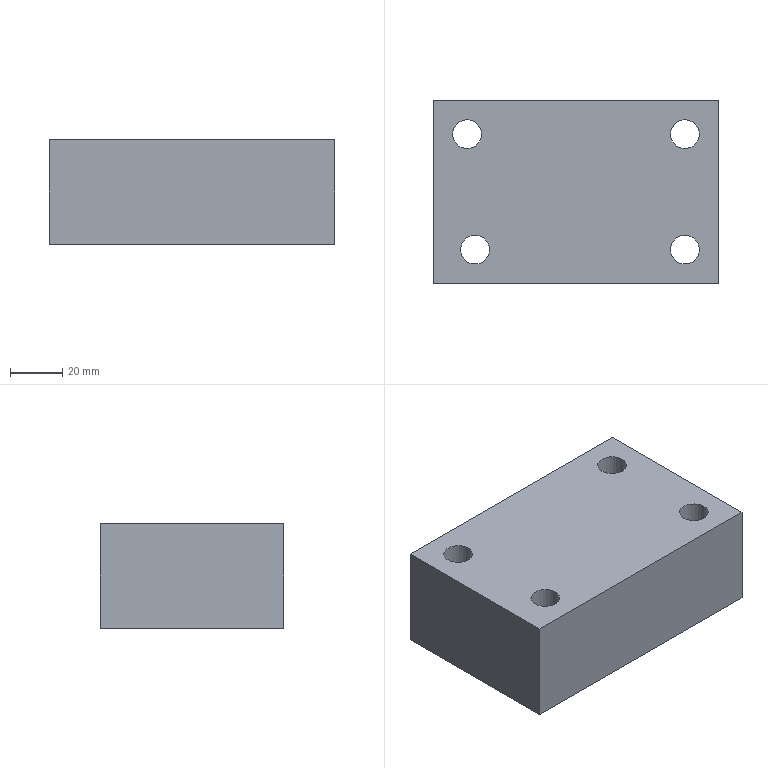Part | STEP file | 119_id1190_x_t | 1 solid | 18 faces | box 109 x 70 x 40 mm | volume 276800 mm3 | plane 10 | cylinder 8 | commonest cylinder face diameters 11 x4 17 x4
STEP:
#1=CARTESIAN_POINT('',(0.,0.,0.));
#2=DIRECTION('',(0.,0.,1.));
#3=DIRECTION('',(1.,0.,0.));
#4=AXIS2_PLACEMENT_3D('',#1,#2,#3);
#5=CARTESIAN_POINT('',(380.5,-156.,65.));
#6=VERTEX_POINT('',#5);
#7=CARTESIAN_POINT('',(380.5,-156.,105.));
#8=VERTEX_POINT('',#7);
#9=CARTESIAN_POINT('',(380.5,-156.,90.));
#10=DIRECTION('',(0.,0.,1.));
#11=VECTOR('',#10,1.);
#12=LINE('',#9,#11);
#13=CARTESIAN_POINT('',(325.,-156.,90.));
#14=DIRECTION('',(0.,-1.,0.));
#15=DIRECTION('',(0.,0.,1.));
#16=AXIS2_PLACEMENT_3D('',#13,#14,#15);
#17=PLANE('',#16);
#18=CARTESIAN_POINT('',(0.,-55.5));
#19=DIRECTION('',(1.,0.));
#20=VECTOR('',#19,1.);
#21=LINE('',#18,#20);
#22=(GEOMETRIC_REPRESENTATION_CONTEXT(2)PARAMETRIC_REPRESENTATION_CONTEXT()REPRESENTATION_CONTEXT('',''));
#23=DEFINITIONAL_REPRESENTATION('',(#21),#22);
#24=PCURVE('',#17,#23);
#25=CARTESIAN_POINT('',(380.5,-122.5,90.));
#26=DIRECTION('',(1.,0.,0.));
#27=DIRECTION('',(0.,0.,1.));
#28=AXIS2_PLACEMENT_3D('',#25,#26,#27);
#29=PLANE('',#28);
#30=CARTESIAN_POINT('',(0.,33.5));
#31=DIRECTION('',(1.,0.));
#32=VECTOR('',#31,1.);
#33=LINE('',#30,#32);
#34=(GEOMETRIC_REPRESENTATION_CONTEXT(2)PARAMETRIC_REPRESENTATION_CONTEXT()REPRESENTATION_CONTEXT('',''));
#35=DEFINITIONAL_REPRESENTATION('',(#33),#34);
#36=PCURVE('',#29,#35);
#37=SURFACE_CURVE('',#12,(#24,#36),.PCURVE_S1.);
#38=EDGE_CURVE('',#6,#8,#37,.T.);
#39=ORIENTED_EDGE('',*,*,#38,.T.);
#40=CARTESIAN_POINT('',(271.5,-156.,105.));
#41=VERTEX_POINT('',#40);
#42=CARTESIAN_POINT('',(325.,-156.,105.));
#43=DIRECTION('',(-1.,0.,0.));
#44=VECTOR('',#43,1.);
#45=LINE('',#42,#44);
#46=CARTESIAN_POINT('',(15.,0.));
#47=DIRECTION('',(0.,1.));
#48=VECTOR('',#47,1.);
#49=LINE('',#46,#48);
#50=(GEOMETRIC_REPRESENTATION_CONTEXT(2)PARAMETRIC_REPRESENTATION_CONTEXT()REPRESENTATION_CONTEXT('',''));
#51=DEFINITIONAL_REPRESENTATION('',(#49),#50);
#52=PCURVE('',#17,#51);
#53=CARTESIAN_POINT('',(325.,-122.5,105.));
#54=DIRECTION('',(0.,0.,1.));
#55=DIRECTION('',(-1.,0.,0.));
#56=AXIS2_PLACEMENT_3D('',#53,#54,#55);
#57=PLANE('',#56);
#58=CARTESIAN_POINT('',(0.,33.5));
#59=DIRECTION('',(1.,0.));
#60=VECTOR('',#59,1.);
#61=LINE('',#58,#60);
#62=(GEOMETRIC_REPRESENTATION_CONTEXT(2)PARAMETRIC_REPRESENTATION_CONTEXT()REPRESENTATION_CONTEXT('',''));
#63=DEFINITIONAL_REPRESENTATION('',(#61),#62);
#64=PCURVE('',#57,#63);
#65=SURFACE_CURVE('',#45,(#52,#64),.PCURVE_S1.);
#66=EDGE_CURVE('',#8,#41,#65,.T.);
#67=ORIENTED_EDGE('',*,*,#66,.T.);
#68=CARTESIAN_POINT('',(271.5,-156.,65.));
#69=VERTEX_POINT('',#68);
#70=CARTESIAN_POINT('',(271.5,-156.,90.));
#71=DIRECTION('',(0.,0.,1.));
#72=VECTOR('',#71,1.);
#73=LINE('',#70,#72);
#74=CARTESIAN_POINT('',(0.,53.5));
#75=DIRECTION('',(1.,0.));
#76=VECTOR('',#75,1.);
#77=LINE('',#74,#76);
#78=(GEOMETRIC_REPRESENTATION_CONTEXT(2)PARAMETRIC_REPRESENTATION_CONTEXT()REPRESENTATION_CONTEXT('',''));
#79=DEFINITIONAL_REPRESENTATION('',(#77),#78);
#80=PCURVE('',#17,#79);
#81=CARTESIAN_POINT('',(271.5,-122.5,90.));
#82=DIRECTION('',(-1.,0.,0.));
#83=DIRECTION('',(0.,0.,-1.));
#84=AXIS2_PLACEMENT_3D('',#81,#82,#83);
#85=PLANE('',#84);
#86=CARTESIAN_POINT('',(0.,33.5));
#87=DIRECTION('',(-1.,0.));
#88=VECTOR('',#87,1.);
#89=LINE('',#86,#88);
#90=(GEOMETRIC_REPRESENTATION_CONTEXT(2)PARAMETRIC_REPRESENTATION_CONTEXT()REPRESENTATION_CONTEXT('',''));
#91=DEFINITIONAL_REPRESENTATION('',(#89),#90);
#92=PCURVE('',#85,#91);
#93=SURFACE_CURVE('',#73,(#80,#92),.PCURVE_S1.);
#94=EDGE_CURVE('',#69,#41,#93,.T.);
#95=ORIENTED_EDGE('',*,*,#94,.F.);
#96=CARTESIAN_POINT('',(325.,-156.,65.));
#97=DIRECTION('',(1.,0.,0.));
#98=VECTOR('',#97,1.);
#99=LINE('',#96,#98);
#100=CARTESIAN_POINT('',(-25.,0.));
#101=DIRECTION('',(0.,-1.));
#102=VECTOR('',#101,1.);
#103=LINE('',#100,#102);
#104=(GEOMETRIC_REPRESENTATION_CONTEXT(2)PARAMETRIC_REPRESENTATION_CONTEXT()REPRESENTATION_CONTEXT('',''));
#105=DEFINITIONAL_REPRESENTATION('',(#103),#104);
#106=PCURVE('',#17,#105);
#107=CARTESIAN_POINT('',(-346.389,-676.223,65.));
#108=DIRECTION('',(0.,0.,-1.));
#109=DIRECTION('',(-1.,0.,0.));
#110=AXIS2_PLACEMENT_3D('',#107,#108,#109);
#111=PLANE('',#110);
#112=CARTESIAN_POINT('',(-671.389,520.223));
#113=DIRECTION('',(-1.,0.));
#114=VECTOR('',#113,1.);
#115=LINE('',#112,#114);
#116=(GEOMETRIC_REPRESENTATION_CONTEXT(2)PARAMETRIC_REPRESENTATION_CONTEXT()REPRESENTATION_CONTEXT('',''));
#117=DEFINITIONAL_REPRESENTATION('',(#115),#116);
#118=PCURVE('',#111,#117);
#119=SURFACE_CURVE('',#99,(#106,#118),.PCURVE_S1.);
#120=EDGE_CURVE('',#69,#6,#119,.T.);
#121=ORIENTED_EDGE('',*,*,#120,.T.);
#122=EDGE_LOOP('',(#39,#67,#95,#121));
#123=FACE_BOUND('',#122,.T.);
#124=ADVANCED_FACE('',(#123),#17,.T.);
#125=ORIENTED_EDGE('',*,*,#94,.T.);
#126=CARTESIAN_POINT('',(271.5,-86.,105.));
#127=VERTEX_POINT('',#126);
#128=CARTESIAN_POINT('',(271.5,-122.5,105.));
#129=DIRECTION('',(0.,1.,0.));
#130=VECTOR('',#129,1.);
#131=LINE('',#128,#130);
#132=CARTESIAN_POINT('',(-15.,0.));
#133=DIRECTION('',(0.,-1.));
#134=VECTOR('',#133,1.);
#135=LINE('',#132,#134);
#136=(GEOMETRIC_REPRESENTATION_CONTEXT(2)PARAMETRIC_REPRESENTATION_CONTEXT()REPRESENTATION_CONTEXT('',''));
#137=DEFINITIONAL_REPRESENTATION('',(#135),#136);
#138=PCURVE('',#85,#137);
#139=CARTESIAN_POINT('',(53.5,0.));
#140=DIRECTION('',(0.,-1.));
#141=VECTOR('',#140,1.);
#142=LINE('',#139,#141);
#143=(GEOMETRIC_REPRESENTATION_CONTEXT(2)PARAMETRIC_REPRESENTATION_CONTEXT()REPRESENTATION_CONTEXT('',''));
#144=DEFINITIONAL_REPRESENTATION('',(#142),#143);
#145=PCURVE('',#57,#144);
#146=SURFACE_CURVE('',#131,(#138,#145),.PCURVE_S1.);
#147=EDGE_CURVE('',#41,#127,#146,.T.);
#148=ORIENTED_EDGE('',*,*,#147,.T.);
#149=CARTESIAN_POINT('',(271.5,-86.,65.));
#150=VERTEX_POINT('',#149);
#151=CARTESIAN_POINT('',(271.5,-86.,90.));
#152=DIRECTION('',(0.,0.,1.));
#153=VECTOR('',#152,1.);
#154=LINE('',#151,#153);
#155=CARTESIAN_POINT('',(0.,-36.5));
#156=DIRECTION('',(-1.,0.));
#157=VECTOR('',#156,1.);
#158=LINE('',#155,#157);
#159=(GEOMETRIC_REPRESENTATION_CONTEXT(2)PARAMETRIC_REPRESENTATION_CONTEXT()REPRESENTATION_CONTEXT('',''));
#160=DEFINITIONAL_REPRESENTATION('',(#158),#159);
#161=PCURVE('',#85,#160);
#162=CARTESIAN_POINT('',(325.,-86.,90.));
#163=DIRECTION('',(0.,1.,0.));
#164=DIRECTION('',(0.,0.,-1.));
#165=AXIS2_PLACEMENT_3D('',#162,#163,#164);
#166=PLANE('',#165);
#167=CARTESIAN_POINT('',(0.,53.5));
#168=DIRECTION('',(-1.,0.));
#169=VECTOR('',#168,1.);
#170=LINE('',#167,#169);
#171=(GEOMETRIC_REPRESENTATION_CONTEXT(2)PARAMETRIC_REPRESENTATION_CONTEXT()REPRESENTATION_CONTEXT('',''));
#172=DEFINITIONAL_REPRESENTATION('',(#170),#171);
#173=PCURVE('',#166,#172);
#174=SURFACE_CURVE('',#154,(#161,#173),.PCURVE_S1.);
#175=EDGE_CURVE('',#150,#127,#174,.T.);
#176=ORIENTED_EDGE('',*,*,#175,.F.);
#177=CARTESIAN_POINT('',(271.5,-122.5,65.));
#178=DIRECTION('',(0.,-1.,0.));
#179=VECTOR('',#178,1.);
#180=LINE('',#177,#179);
#181=CARTESIAN_POINT('',(25.,0.));
#182=DIRECTION('',(0.,1.));
#183=VECTOR('',#182,1.);
#184=LINE('',#181,#183);
#185=(GEOMETRIC_REPRESENTATION_CONTEXT(2)PARAMETRIC_REPRESENTATION_CONTEXT()REPRESENTATION_CONTEXT('',''));
#186=DEFINITIONAL_REPRESENTATION('',(#184),#185);
#187=PCURVE('',#85,#186);
#188=CARTESIAN_POINT('',(-617.889,553.723));
#189=DIRECTION('',(0.,-1.));
#190=VECTOR('',#189,1.);
#191=LINE('',#188,#190);
#192=(GEOMETRIC_REPRESENTATION_CONTEXT(2)PARAMETRIC_REPRESENTATION_CONTEXT()REPRESENTATION_CONTEXT('',''));
#193=DEFINITIONAL_REPRESENTATION('',(#191),#192);
#194=PCURVE('',#111,#193);
#195=SURFACE_CURVE('',#180,(#187,#194),.PCURVE_S1.);
#196=EDGE_CURVE('',#150,#69,#195,.T.);
#197=ORIENTED_EDGE('',*,*,#196,.T.);
#198=EDGE_LOOP('',(#125,#148,#176,#197));
#199=FACE_BOUND('',#198,.T.);
#200=ADVANCED_FACE('',(#199),#85,.T.);
#201=ORIENTED_EDGE('',*,*,#175,.T.);
#202=CARTESIAN_POINT('',(380.5,-86.,105.));
#203=VERTEX_POINT('',#202);
#204=CARTESIAN_POINT('',(325.,-86.,105.));
#205=DIRECTION('',(1.,0.,0.));
#206=VECTOR('',#205,1.);
#207=LINE('',#204,#206);
#208=CARTESIAN_POINT('',(-15.,0.));
#209=DIRECTION('',(0.,-1.));
#210=VECTOR('',#209,1.);
#211=LINE('',#208,#210);
#212=(GEOMETRIC_REPRESENTATION_CONTEXT(2)PARAMETRIC_REPRESENTATION_CONTEXT()REPRESENTATION_CONTEXT('',''));
#213=DEFINITIONAL_REPRESENTATION('',(#211),#212);
#214=PCURVE('',#166,#213);
#215=CARTESIAN_POINT('',(0.,-36.5));
#216=DIRECTION('',(-1.,0.));
#217=VECTOR('',#216,1.);
#218=LINE('',#215,#217);
#219=(GEOMETRIC_REPRESENTATION_CONTEXT(2)PARAMETRIC_REPRESENTATION_CONTEXT()REPRESENTATION_CONTEXT('',''));
#220=DEFINITIONAL_REPRESENTATION('',(#218),#219);
#221=PCURVE('',#57,#220);
#222=SURFACE_CURVE('',#207,(#214,#221),.PCURVE_S1.);
#223=EDGE_CURVE('',#127,#203,#222,.T.);
#224=ORIENTED_EDGE('',*,*,#223,.T.);
#225=CARTESIAN_POINT('',(380.5,-86.,65.));
#226=VERTEX_POINT('',#225);
#227=CARTESIAN_POINT('',(380.5,-86.,90.));
#228=DIRECTION('',(0.,0.,1.));
#229=VECTOR('',#228,1.);
#230=LINE('',#227,#229);
#231=CARTESIAN_POINT('',(0.,-55.5));
#232=DIRECTION('',(-1.,0.));
#233=VECTOR('',#232,1.);
#234=LINE('',#231,#233);
#235=(GEOMETRIC_REPRESENTATION_CONTEXT(2)PARAMETRIC_REPRESENTATION_CONTEXT()REPRESENTATION_CONTEXT('',''));
#236=DEFINITIONAL_REPRESENTATION('',(#234),#235);
#237=PCURVE('',#166,#236);
#238=CARTESIAN_POINT('',(0.,-36.5));
#239=DIRECTION('',(1.,0.));
#240=VECTOR('',#239,1.);
#241=LINE('',#238,#240);
#242=(GEOMETRIC_REPRESENTATION_CONTEXT(2)PARAMETRIC_REPRESENTATION_CONTEXT()REPRESENTATION_CONTEXT('',''));
#243=DEFINITIONAL_REPRESENTATION('',(#241),#242);
#244=PCURVE('',#29,#243);
#245=SURFACE_CURVE('',#230,(#237,#244),.PCURVE_S1.);
#246=EDGE_CURVE('',#226,#203,#245,.T.);
#247=ORIENTED_EDGE('',*,*,#246,.F.);
#248=CARTESIAN_POINT('',(325.,-86.,65.));
#249=DIRECTION('',(-1.,0.,0.));
#250=VECTOR('',#249,1.);
#251=LINE('',#248,#250);
#252=CARTESIAN_POINT('',(25.,0.));
#253=DIRECTION('',(0.,1.));
#254=VECTOR('',#253,1.);
#255=LINE('',#252,#254);
#256=(GEOMETRIC_REPRESENTATION_CONTEXT(2)PARAMETRIC_REPRESENTATION_CONTEXT()REPRESENTATION_CONTEXT('',''));
#257=DEFINITIONAL_REPRESENTATION('',(#255),#256);
#258=PCURVE('',#166,#257);
#259=CARTESIAN_POINT('',(-671.389,590.223));
#260=DIRECTION('',(1.,0.));
#261=VECTOR('',#260,1.);
#262=LINE('',#259,#261);
#263=(GEOMETRIC_REPRESENTATION_CONTEXT(2)PARAMETRIC_REPRESENTATION_CONTEXT()REPRESENTATION_CONTEXT('',''));
#264=DEFINITIONAL_REPRESENTATION('',(#262),#263);
#265=PCURVE('',#111,#264);
#266=SURFACE_CURVE('',#251,(#258,#265),.PCURVE_S1.);
#267=EDGE_CURVE('',#226,#150,#266,.T.);
#268=ORIENTED_EDGE('',*,*,#267,.T.);
#269=EDGE_LOOP('',(#201,#224,#247,#268));
#270=FACE_BOUND('',#269,.T.);
#271=ADVANCED_FACE('',(#270),#166,.T.);
#272=ORIENTED_EDGE('',*,*,#246,.T.);
#273=CARTESIAN_POINT('',(380.5,-122.5,105.));
#274=DIRECTION('',(0.,-1.,0.));
#275=VECTOR('',#274,1.);
#276=LINE('',#273,#275);
#277=CARTESIAN_POINT('',(15.,0.));
#278=DIRECTION('',(0.,1.));
#279=VECTOR('',#278,1.);
#280=LINE('',#277,#279);
#281=(GEOMETRIC_REPRESENTATION_CONTEXT(2)PARAMETRIC_REPRESENTATION_CONTEXT()REPRESENTATION_CONTEXT('',''));
#282=DEFINITIONAL_REPRESENTATION('',(#280),#281);
#283=PCURVE('',#29,#282);
#284=CARTESIAN_POINT('',(-55.5,0.));
#285=DIRECTION('',(0.,1.));
#286=VECTOR('',#285,1.);
#287=LINE('',#284,#286);
#288=(GEOMETRIC_REPRESENTATION_CONTEXT(2)PARAMETRIC_REPRESENTATION_CONTEXT()REPRESENTATION_CONTEXT('',''));
#289=DEFINITIONAL_REPRESENTATION('',(#287),#288);
#290=PCURVE('',#57,#289);
#291=SURFACE_CURVE('',#276,(#283,#290),.PCURVE_S1.);
#292=EDGE_CURVE('',#203,#8,#291,.T.);
#293=ORIENTED_EDGE('',*,*,#292,.T.);
#294=ORIENTED_EDGE('',*,*,#38,.F.);
#295=CARTESIAN_POINT('',(380.5,-122.5,65.));
#296=DIRECTION('',(0.,1.,0.));
#297=VECTOR('',#296,1.);
#298=LINE('',#295,#297);
#299=CARTESIAN_POINT('',(-25.,0.));
#300=DIRECTION('',(0.,-1.));
#301=VECTOR('',#300,1.);
#302=LINE('',#299,#301);
#303=(GEOMETRIC_REPRESENTATION_CONTEXT(2)PARAMETRIC_REPRESENTATION_CONTEXT()REPRESENTATION_CONTEXT('',''));
#304=DEFINITIONAL_REPRESENTATION('',(#302),#303);
#305=PCURVE('',#29,#304);
#306=CARTESIAN_POINT('',(-726.889,553.723));
#307=DIRECTION('',(0.,1.));
#308=VECTOR('',#307,1.);
#309=LINE('',#306,#308);
#310=(GEOMETRIC_REPRESENTATION_CONTEXT(2)PARAMETRIC_REPRESENTATION_CONTEXT()REPRESENTATION_CONTEXT('',''));
#311=DEFINITIONAL_REPRESENTATION('',(#309),#310);
#312=PCURVE('',#111,#311);
#313=SURFACE_CURVE('',#298,(#305,#312),.PCURVE_S1.);
#314=EDGE_CURVE('',#6,#226,#313,.T.);
#315=ORIENTED_EDGE('',*,*,#314,.T.);
#316=EDGE_LOOP('',(#272,#293,#294,#315));
#317=FACE_BOUND('',#316,.T.);
#318=ADVANCED_FACE('',(#317),#29,.T.);
#319=CARTESIAN_POINT('',(279.,-143.,65.));
#320=VERTEX_POINT('',#319);
#321=CARTESIAN_POINT('',(287.5,-143.,65.));
#322=DIRECTION('',(0.,0.,1.));
#323=DIRECTION('',(-1.,0.,0.));
#324=AXIS2_PLACEMENT_3D('',#321,#322,#323);
#325=CIRCLE('',#324,8.5);
#326=CARTESIAN_POINT('',(287.5,-143.,90.));
#327=DIRECTION('',(0.,0.,1.));
#328=DIRECTION('',(-1.,0.,0.));
#329=AXIS2_PLACEMENT_3D('',#326,#327,#328);
#330=CYLINDRICAL_SURFACE('',#329,8.5);
#331=CARTESIAN_POINT('',(0.,-25.));
#332=DIRECTION('',(1.,0.));
#333=VECTOR('',#332,1.);
#334=LINE('',#331,#333);
#335=(GEOMETRIC_REPRESENTATION_CONTEXT(2)PARAMETRIC_REPRESENTATION_CONTEXT()REPRESENTATION_CONTEXT('',''));
#336=DEFINITIONAL_REPRESENTATION('',(#334),#335);
#337=PCURVE('',#330,#336);
#338=CARTESIAN_POINT('',(-625.389,533.223));
#339=CARTESIAN_POINT('',(-625.389,518.5));
#340=CARTESIAN_POINT('',(-638.139,525.862));
#341=CARTESIAN_POINT('',(-650.889,533.223));
#342=CARTESIAN_POINT('',(-638.139,540.584));
#343=CARTESIAN_POINT('',(-625.389,547.945));
#344=CARTESIAN_POINT('',(-625.389,533.223));
#345=(BOUNDED_CURVE()B_SPLINE_CURVE(2,(#338,#339,#340,#341,#342,#343,#344),.UNSPECIFIED.,.T.,.F.)B_SPLINE_CURVE_WITH_KNOTS((1,2,2,2,2,1),(-2.094,0.,2.094,4.189,6.283,8.378),.UNSPECIFIED.)CURVE()GEOMETRIC_REPRESENTATION_ITEM()RATIONAL_B_SPLINE_CURVE((1.,0.5,1.,0.5,1.,0.5,1.))REPRESENTATION_ITEM(''));
#346=(GEOMETRIC_REPRESENTATION_CONTEXT(2)PARAMETRIC_REPRESENTATION_CONTEXT()REPRESENTATION_CONTEXT('',''));
#347=DEFINITIONAL_REPRESENTATION('',(#345),#346);
#348=PCURVE('',#111,#347);
#349=SURFACE_CURVE('',#325,(#337,#348),.PCURVE_S1.);
#350=EDGE_CURVE('',#320,#320,#349,.T.);
#351=ORIENTED_EDGE('',*,*,#350,.T.);
#352=CARTESIAN_POINT('',(279.,-143.,90.));
#353=VERTEX_POINT('',#352);
#354=CARTESIAN_POINT('',(279.,-143.,65.));
#355=CARTESIAN_POINT('',(279.,-143.,90.));
#356=B_SPLINE_CURVE_WITH_KNOTS('',1,(#354,#355),.UNSPECIFIED.,.F.,.F.,(2,2),(-25.,0.),.PIECEWISE_BEZIER_KNOTS.);
#357=CARTESIAN_POINT('',(6.283,0.));
#358=DIRECTION('',(0.,1.));
#359=VECTOR('',#358,1.);
#360=LINE('',#357,#359);
#361=(GEOMETRIC_REPRESENTATION_CONTEXT(2)PARAMETRIC_REPRESENTATION_CONTEXT()REPRESENTATION_CONTEXT('',''));
#362=DEFINITIONAL_REPRESENTATION('',(#360),#361);
#363=PCURVE('',#330,#362);
#364=CARTESIAN_POINT('',(0.,0.));
#365=DIRECTION('',(0.,1.));
#366=VECTOR('',#365,1.);
#367=LINE('',#364,#366);
#368=(GEOMETRIC_REPRESENTATION_CONTEXT(2)PARAMETRIC_REPRESENTATION_CONTEXT()REPRESENTATION_CONTEXT('',''));
#369=DEFINITIONAL_REPRESENTATION('',(#367),#368);
#370=PCURVE('',#330,#369);
#371=SEAM_CURVE('',#356,(#363,#370),.PCURVE_S1.);
#372=EDGE_CURVE('',#320,#353,#371,.T.);
#373=ORIENTED_EDGE('',*,*,#372,.T.);
#374=CARTESIAN_POINT('',(296.,-143.,90.));
#375=VERTEX_POINT('',#374);
#376=CARTESIAN_POINT('',(287.5,-143.,90.));
#377=DIRECTION('',(0.,0.,1.));
#378=DIRECTION('',(1.,0.,0.));
#379=AXIS2_PLACEMENT_3D('',#376,#377,#378);
#380=CIRCLE('',#379,8.5);
#381=CARTESIAN_POINT('',(3.142,0.));
#382=DIRECTION('',(1.,0.));
#383=VECTOR('',#382,1.);
#384=LINE('',#381,#383);
#385=(GEOMETRIC_REPRESENTATION_CONTEXT(2)PARAMETRIC_REPRESENTATION_CONTEXT()REPRESENTATION_CONTEXT('',''));
#386=DEFINITIONAL_REPRESENTATION('',(#384),#385);
#387=PCURVE('',#330,#386);
#388=CARTESIAN_POINT('',(326.,-121.,90.));
#389=DIRECTION('',(0.,0.,1.));
#390=DIRECTION('',(1.,0.,0.));
#391=AXIS2_PLACEMENT_3D('',#388,#389,#390);
#392=PLANE('',#391);
#393=CARTESIAN_POINT('',(-38.5,-22.));
#394=DIRECTION('',(1.,0.));
#395=AXIS2_PLACEMENT_2D('',#393,#394);
#396=CIRCLE('',#395,8.5);
#397=(GEOMETRIC_REPRESENTATION_CONTEXT(2)PARAMETRIC_REPRESENTATION_CONTEXT()REPRESENTATION_CONTEXT('',''));
#398=DEFINITIONAL_REPRESENTATION('',(#396),#397);
#399=PCURVE('',#392,#398);
#400=SURFACE_CURVE('',#380,(#387,#399),.PCURVE_S1.);
#401=EDGE_CURVE('',#375,#353,#400,.T.);
#402=ORIENTED_EDGE('',*,*,#401,.F.);
#403=CARTESIAN_POINT('',(287.5,-143.,90.));
#404=DIRECTION('',(0.,0.,1.));
#405=DIRECTION('',(1.,0.,0.));
#406=AXIS2_PLACEMENT_3D('',#403,#404,#405);
#407=CIRCLE('',#406,8.5);
#408=CARTESIAN_POINT('',(-3.142,0.));
#409=DIRECTION('',(1.,0.));
#410=VECTOR('',#409,1.);
#411=LINE('',#408,#410);
#412=(GEOMETRIC_REPRESENTATION_CONTEXT(2)PARAMETRIC_REPRESENTATION_CONTEXT()REPRESENTATION_CONTEXT('',''));
#413=DEFINITIONAL_REPRESENTATION('',(#411),#412);
#414=PCURVE('',#330,#413);
#415=CARTESIAN_POINT('',(-38.5,-22.));
#416=DIRECTION('',(1.,0.));
#417=AXIS2_PLACEMENT_2D('',#415,#416);
#418=CIRCLE('',#417,8.5);
#419=(GEOMETRIC_REPRESENTATION_CONTEXT(2)PARAMETRIC_REPRESENTATION_CONTEXT()REPRESENTATION_CONTEXT('',''));
#420=DEFINITIONAL_REPRESENTATION('',(#418),#419);
#421=PCURVE('',#392,#420);
#422=SURFACE_CURVE('',#407,(#414,#421),.PCURVE_S1.);
#423=EDGE_CURVE('',#353,#375,#422,.T.);
#424=ORIENTED_EDGE('',*,*,#423,.F.);
#425=ORIENTED_EDGE('',*,*,#372,.F.);
#426=EDGE_LOOP('',(#351,#373,#402,#424,#425));
#427=FACE_BOUND('',#426,.F.);
#428=ADVANCED_FACE('',(#427),#330,.F.);
#429=CARTESIAN_POINT('',(359.,-143.,65.));
#430=VERTEX_POINT('',#429);
#431=CARTESIAN_POINT('',(367.5,-143.,65.));
#432=DIRECTION('',(0.,0.,1.));
#433=DIRECTION('',(-1.,0.,0.));
#434=AXIS2_PLACEMENT_3D('',#431,#432,#433);
#435=CIRCLE('',#434,8.5);
#436=CARTESIAN_POINT('',(367.5,-143.,90.));
#437=DIRECTION('',(0.,0.,1.));
#438=DIRECTION('',(-1.,0.,0.));
#439=AXIS2_PLACEMENT_3D('',#436,#437,#438);
#440=CYLINDRICAL_SURFACE('',#439,8.5);
#441=CARTESIAN_POINT('',(0.,-25.));
#442=DIRECTION('',(1.,0.));
#443=VECTOR('',#442,1.);
#444=LINE('',#441,#443);
#445=(GEOMETRIC_REPRESENTATION_CONTEXT(2)PARAMETRIC_REPRESENTATION_CONTEXT()REPRESENTATION_CONTEXT('',''));
#446=DEFINITIONAL_REPRESENTATION('',(#444),#445);
#447=PCURVE('',#440,#446);
#448=CARTESIAN_POINT('',(-705.389,533.223));
#449=CARTESIAN_POINT('',(-705.389,518.5));
#450=CARTESIAN_POINT('',(-718.139,525.862));
#451=CARTESIAN_POINT('',(-730.889,533.223));
#452=CARTESIAN_POINT('',(-718.139,540.584));
#453=CARTESIAN_POINT('',(-705.389,547.945));
#454=CARTESIAN_POINT('',(-705.389,533.223));
#455=(BOUNDED_CURVE()B_SPLINE_CURVE(2,(#448,#449,#450,#451,#452,#453,#454),.UNSPECIFIED.,.T.,.F.)B_SPLINE_CURVE_WITH_KNOTS((1,2,2,2,2,1),(-2.094,0.,2.094,4.189,6.283,8.378),.UNSPECIFIED.)CURVE()GEOMETRIC_REPRESENTATION_ITEM()RATIONAL_B_SPLINE_CURVE((1.,0.5,1.,0.5,1.,0.5,1.))REPRESENTATION_ITEM(''));
#456=(GEOMETRIC_REPRESENTATION_CONTEXT(2)PARAMETRIC_REPRESENTATION_CONTEXT()REPRESENTATION_CONTEXT('',''));
#457=DEFINITIONAL_REPRESENTATION('',(#455),#456);
#458=PCURVE('',#111,#457);
#459=SURFACE_CURVE('',#435,(#447,#458),.PCURVE_S1.);
#460=EDGE_CURVE('',#430,#430,#459,.T.);
#461=ORIENTED_EDGE('',*,*,#460,.T.);
#462=CARTESIAN_POINT('',(359.,-143.,90.));
#463=VERTEX_POINT('',#462);
#464=CARTESIAN_POINT('',(359.,-143.,65.));
#465=CARTESIAN_POINT('',(359.,-143.,90.));
#466=B_SPLINE_CURVE_WITH_KNOTS('',1,(#464,#465),.UNSPECIFIED.,.F.,.F.,(2,2),(-25.,0.),.PIECEWISE_BEZIER_KNOTS.);
#467=CARTESIAN_POINT('',(6.283,0.));
#468=DIRECTION('',(0.,1.));
#469=VECTOR('',#468,1.);
#470=LINE('',#467,#469);
#471=(GEOMETRIC_REPRESENTATION_CONTEXT(2)PARAMETRIC_REPRESENTATION_CONTEXT()REPRESENTATION_CONTEXT('',''));
#472=DEFINITIONAL_REPRESENTATION('',(#470),#471);
#473=PCURVE('',#440,#472);
#474=CARTESIAN_POINT('',(0.,0.));
#475=DIRECTION('',(0.,1.));
#476=VECTOR('',#475,1.);
#477=LINE('',#474,#476);
#478=(GEOMETRIC_REPRESENTATION_CONTEXT(2)PARAMETRIC_REPRESENTATION_CONTEXT()REPRESENTATION_CONTEXT('',''));
#479=DEFINITIONAL_REPRESENTATION('',(#477),#478);
#480=PCURVE('',#440,#479);
#481=SEAM_CURVE('',#466,(#473,#480),.PCURVE_S1.);
#482=EDGE_CURVE('',#430,#463,#481,.T.);
#483=ORIENTED_EDGE('',*,*,#482,.T.);
#484=CARTESIAN_POINT('',(376.,-143.,90.));
#485=VERTEX_POINT('',#484);
#486=CARTESIAN_POINT('',(367.5,-143.,90.));
#487=DIRECTION('',(0.,0.,1.));
#488=DIRECTION('',(1.,0.,0.));
#489=AXIS2_PLACEMENT_3D('',#486,#487,#488);
#490=CIRCLE('',#489,8.5);
#491=CARTESIAN_POINT('',(3.142,0.));
#492=DIRECTION('',(1.,0.));
#493=VECTOR('',#492,1.);
#494=LINE('',#491,#493);
#495=(GEOMETRIC_REPRESENTATION_CONTEXT(2)PARAMETRIC_REPRESENTATION_CONTEXT()REPRESENTATION_CONTEXT('',''));
#496=DEFINITIONAL_REPRESENTATION('',(#494),#495);
#497=PCURVE('',#440,#496);
#498=CARTESIAN_POINT('',(326.,-121.,90.));
#499=DIRECTION('',(0.,0.,1.));
#500=DIRECTION('',(1.,0.,0.));
#501=AXIS2_PLACEMENT_3D('',#498,#499,#500);
#502=PLANE('',#501);
#503=CARTESIAN_POINT('',(41.5,-22.));
#504=DIRECTION('',(1.,0.));
#505=AXIS2_PLACEMENT_2D('',#503,#504);
#506=CIRCLE('',#505,8.5);
#507=(GEOMETRIC_REPRESENTATION_CONTEXT(2)PARAMETRIC_REPRESENTATION_CONTEXT()REPRESENTATION_CONTEXT('',''));
#508=DEFINITIONAL_REPRESENTATION('',(#506),#507);
#509=PCURVE('',#502,#508);
#510=SURFACE_CURVE('',#490,(#497,#509),.PCURVE_S1.);
#511=EDGE_CURVE('',#485,#463,#510,.T.);
#512=ORIENTED_EDGE('',*,*,#511,.F.);
#513=CARTESIAN_POINT('',(367.5,-143.,90.));
#514=DIRECTION('',(0.,0.,1.));
#515=DIRECTION('',(1.,0.,0.));
#516=AXIS2_PLACEMENT_3D('',#513,#514,#515);
#517=CIRCLE('',#516,8.5);
#518=CARTESIAN_POINT('',(-3.142,0.));
#519=DIRECTION('',(1.,0.));
#520=VECTOR('',#519,1.);
#521=LINE('',#518,#520);
#522=(GEOMETRIC_REPRESENTATION_CONTEXT(2)PARAMETRIC_REPRESENTATION_CONTEXT()REPRESENTATION_CONTEXT('',''));
#523=DEFINITIONAL_REPRESENTATION('',(#521),#522);
#524=PCURVE('',#440,#523);
#525=CARTESIAN_POINT('',(41.5,-22.));
#526=DIRECTION('',(1.,0.));
#527=AXIS2_PLACEMENT_2D('',#525,#526);
#528=CIRCLE('',#527,8.5);
#529=(GEOMETRIC_REPRESENTATION_CONTEXT(2)PARAMETRIC_REPRESENTATION_CONTEXT()REPRESENTATION_CONTEXT('',''));
#530=DEFINITIONAL_REPRESENTATION('',(#528),#529);
#531=PCURVE('',#502,#530);
#532=SURFACE_CURVE('',#517,(#524,#531),.PCURVE_S1.);
#533=EDGE_CURVE('',#463,#485,#532,.T.);
#534=ORIENTED_EDGE('',*,*,#533,.F.);
#535=ORIENTED_EDGE('',*,*,#482,.F.);
#536=EDGE_LOOP('',(#461,#483,#512,#534,#535));
#537=FACE_BOUND('',#536,.F.);
#538=ADVANCED_FACE('',(#537),#440,.F.);
#539=CARTESIAN_POINT('',(359.,-99.,65.));
#540=VERTEX_POINT('',#539);
#541=CARTESIAN_POINT('',(367.5,-99.,65.));
#542=DIRECTION('',(0.,0.,1.));
#543=DIRECTION('',(-1.,0.,0.));
#544=AXIS2_PLACEMENT_3D('',#541,#542,#543);
#545=CIRCLE('',#544,8.5);
#546=CARTESIAN_POINT('',(367.5,-99.,90.));
#547=DIRECTION('',(0.,0.,1.));
#548=DIRECTION('',(-1.,0.,0.));
#549=AXIS2_PLACEMENT_3D('',#546,#547,#548);
#550=CYLINDRICAL_SURFACE('',#549,8.5);
#551=CARTESIAN_POINT('',(0.,-25.));
#552=DIRECTION('',(1.,0.));
#553=VECTOR('',#552,1.);
#554=LINE('',#551,#553);
#555=(GEOMETRIC_REPRESENTATION_CONTEXT(2)PARAMETRIC_REPRESENTATION_CONTEXT()REPRESENTATION_CONTEXT('',''));
#556=DEFINITIONAL_REPRESENTATION('',(#554),#555);
#557=PCURVE('',#550,#556);
#558=CARTESIAN_POINT('',(-705.389,577.223));
#559=CARTESIAN_POINT('',(-705.389,562.5));
#560=CARTESIAN_POINT('',(-718.139,569.862));
#561=CARTESIAN_POINT('',(-730.889,577.223));
#562=CARTESIAN_POINT('',(-718.139,584.584));
#563=CARTESIAN_POINT('',(-705.389,591.945));
#564=CARTESIAN_POINT('',(-705.389,577.223));
#565=(BOUNDED_CURVE()B_SPLINE_CURVE(2,(#558,#559,#560,#561,#562,#563,#564),.UNSPECIFIED.,.T.,.F.)B_SPLINE_CURVE_WITH_KNOTS((1,2,2,2,2,1),(-2.094,0.,2.094,4.189,6.283,8.378),.UNSPECIFIED.)CURVE()GEOMETRIC_REPRESENTATION_ITEM()RATIONAL_B_SPLINE_CURVE((1.,0.5,1.,0.5,1.,0.5,1.))REPRESENTATION_ITEM(''));
#566=(GEOMETRIC_REPRESENTATION_CONTEXT(2)PARAMETRIC_REPRESENTATION_CONTEXT()REPRESENTATION_CONTEXT('',''));
#567=DEFINITIONAL_REPRESENTATION('',(#565),#566);
#568=PCURVE('',#111,#567);
#569=SURFACE_CURVE('',#545,(#557,#568),.PCURVE_S1.);
#570=EDGE_CURVE('',#540,#540,#569,.T.);
#571=ORIENTED_EDGE('',*,*,#570,.T.);
#572=CARTESIAN_POINT('',(359.,-99.,90.));
#573=VERTEX_POINT('',#572);
#574=CARTESIAN_POINT('',(359.,-99.,65.));
#575=CARTESIAN_POINT('',(359.,-99.,90.));
#576=B_SPLINE_CURVE_WITH_KNOTS('',1,(#574,#575),.UNSPECIFIED.,.F.,.F.,(2,2),(-25.,0.),.PIECEWISE_BEZIER_KNOTS.);
#577=CARTESIAN_POINT('',(6.283,0.));
#578=DIRECTION('',(0.,1.));
#579=VECTOR('',#578,1.);
#580=LINE('',#577,#579);
#581=(GEOMETRIC_REPRESENTATION_CONTEXT(2)PARAMETRIC_REPRESENTATION_CONTEXT()REPRESENTATION_CONTEXT('',''));
#582=DEFINITIONAL_REPRESENTATION('',(#580),#581);
#583=PCURVE('',#550,#582);
#584=CARTESIAN_POINT('',(0.,0.));
#585=DIRECTION('',(0.,1.));
#586=VECTOR('',#585,1.);
#587=LINE('',#584,#586);
#588=(GEOMETRIC_REPRESENTATION_CONTEXT(2)PARAMETRIC_REPRESENTATION_CONTEXT()REPRESENTATION_CONTEXT('',''));
#589=DEFINITIONAL_REPRESENTATION('',(#587),#588);
#590=PCURVE('',#550,#589);
#591=SEAM_CURVE('',#576,(#583,#590),.PCURVE_S1.);
#592=EDGE_CURVE('',#540,#573,#591,.T.);
#593=ORIENTED_EDGE('',*,*,#592,.T.);
#594=CARTESIAN_POINT('',(376.,-99.,90.));
#595=VERTEX_POINT('',#594);
#596=CARTESIAN_POINT('',(367.5,-99.,90.));
#597=DIRECTION('',(0.,0.,1.));
#598=DIRECTION('',(1.,0.,0.));
#599=AXIS2_PLACEMENT_3D('',#596,#597,#598);
#600=CIRCLE('',#599,8.5);
#601=CARTESIAN_POINT('',(3.142,0.));
#602=DIRECTION('',(1.,0.));
#603=VECTOR('',#602,1.);
#604=LINE('',#601,#603);
#605=(GEOMETRIC_REPRESENTATION_CONTEXT(2)PARAMETRIC_REPRESENTATION_CONTEXT()REPRESENTATION_CONTEXT('',''));
#606=DEFINITIONAL_REPRESENTATION('',(#604),#605);
#607=PCURVE('',#550,#606);
#608=CARTESIAN_POINT('',(326.,-121.,90.));
#609=DIRECTION('',(0.,0.,1.));
#610=DIRECTION('',(1.,0.,0.));
#611=AXIS2_PLACEMENT_3D('',#608,#609,#610);
#612=PLANE('',#611);
#613=CARTESIAN_POINT('',(41.5,22.));
#614=DIRECTION('',(1.,0.));
#615=AXIS2_PLACEMENT_2D('',#613,#614);
#616=CIRCLE('',#615,8.5);
#617=(GEOMETRIC_REPRESENTATION_CONTEXT(2)PARAMETRIC_REPRESENTATION_CONTEXT()REPRESENTATION_CONTEXT('',''));
#618=DEFINITIONAL_REPRESENTATION('',(#616),#617);
#619=PCURVE('',#612,#618);
#620=SURFACE_CURVE('',#600,(#607,#619),.PCURVE_S1.);
#621=EDGE_CURVE('',#595,#573,#620,.T.);
#622=ORIENTED_EDGE('',*,*,#621,.F.);
#623=CARTESIAN_POINT('',(367.5,-99.,90.));
#624=DIRECTION('',(0.,0.,1.));
#625=DIRECTION('',(1.,0.,0.));
#626=AXIS2_PLACEMENT_3D('',#623,#624,#625);
#627=CIRCLE('',#626,8.5);
#628=CARTESIAN_POINT('',(-3.142,0.));
#629=DIRECTION('',(1.,0.));
#630=VECTOR('',#629,1.);
#631=LINE('',#628,#630);
#632=(GEOMETRIC_REPRESENTATION_CONTEXT(2)PARAMETRIC_REPRESENTATION_CONTEXT()REPRESENTATION_CONTEXT('',''));
#633=DEFINITIONAL_REPRESENTATION('',(#631),#632);
#634=PCURVE('',#550,#633);
#635=CARTESIAN_POINT('',(41.5,22.));
#636=DIRECTION('',(1.,0.));
#637=AXIS2_PLACEMENT_2D('',#635,#636);
#638=CIRCLE('',#637,8.5);
#639=(GEOMETRIC_REPRESENTATION_CONTEXT(2)PARAMETRIC_REPRESENTATION_CONTEXT()REPRESENTATION_CONTEXT('',''));
#640=DEFINITIONAL_REPRESENTATION('',(#638),#639);
#641=PCURVE('',#612,#640);
#642=SURFACE_CURVE('',#627,(#634,#641),.PCURVE_S1.);
#643=EDGE_CURVE('',#573,#595,#642,.T.);
#644=ORIENTED_EDGE('',*,*,#643,.F.);
#645=ORIENTED_EDGE('',*,*,#592,.F.);
#646=EDGE_LOOP('',(#571,#593,#622,#644,#645));
#647=FACE_BOUND('',#646,.F.);
#648=ADVANCED_FACE('',(#647),#550,.F.);
#649=CARTESIAN_POINT('',(276.,-99.,65.));
#650=VERTEX_POINT('',#649);
#651=CARTESIAN_POINT('',(284.5,-99.,65.));
#652=DIRECTION('',(0.,0.,1.));
#653=DIRECTION('',(-1.,0.,0.));
#654=AXIS2_PLACEMENT_3D('',#651,#652,#653);
#655=CIRCLE('',#654,8.5);
#656=CARTESIAN_POINT('',(284.5,-99.,90.));
#657=DIRECTION('',(0.,0.,1.));
#658=DIRECTION('',(-1.,0.,0.));
#659=AXIS2_PLACEMENT_3D('',#656,#657,#658);
#660=CYLINDRICAL_SURFACE('',#659,8.5);
#661=CARTESIAN_POINT('',(0.,-25.));
#662=DIRECTION('',(1.,0.));
#663=VECTOR('',#662,1.);
#664=LINE('',#661,#663);
#665=(GEOMETRIC_REPRESENTATION_CONTEXT(2)PARAMETRIC_REPRESENTATION_CONTEXT()REPRESENTATION_CONTEXT('',''));
#666=DEFINITIONAL_REPRESENTATION('',(#664),#665);
#667=PCURVE('',#660,#666);
#668=CARTESIAN_POINT('',(-622.389,577.223));
#669=CARTESIAN_POINT('',(-622.389,562.5));
#670=CARTESIAN_POINT('',(-635.139,569.862));
#671=CARTESIAN_POINT('',(-647.889,577.223));
#672=CARTESIAN_POINT('',(-635.139,584.584));
#673=CARTESIAN_POINT('',(-622.389,591.945));
#674=CARTESIAN_POINT('',(-622.389,577.223));
#675=(BOUNDED_CURVE()B_SPLINE_CURVE(2,(#668,#669,#670,#671,#672,#673,#674),.UNSPECIFIED.,.T.,.F.)B_SPLINE_CURVE_WITH_KNOTS((1,2,2,2,2,1),(-2.094,0.,2.094,4.189,6.283,8.378),.UNSPECIFIED.)CURVE()GEOMETRIC_REPRESENTATION_ITEM()RATIONAL_B_SPLINE_CURVE((1.,0.5,1.,0.5,1.,0.5,1.))REPRESENTATION_ITEM(''));
#676=(GEOMETRIC_REPRESENTATION_CONTEXT(2)PARAMETRIC_REPRESENTATION_CONTEXT()REPRESENTATION_CONTEXT('',''));
#677=DEFINITIONAL_REPRESENTATION('',(#675),#676);
#678=PCURVE('',#111,#677);
#679=SURFACE_CURVE('',#655,(#667,#678),.PCURVE_S1.);
#680=EDGE_CURVE('',#650,#650,#679,.T.);
#681=ORIENTED_EDGE('',*,*,#680,.T.);
#682=CARTESIAN_POINT('',(276.,-99.,90.));
#683=VERTEX_POINT('',#682);
#684=CARTESIAN_POINT('',(276.,-99.,65.));
#685=CARTESIAN_POINT('',(276.,-99.,90.));
#686=B_SPLINE_CURVE_WITH_KNOTS('',1,(#684,#685),.UNSPECIFIED.,.F.,.F.,(2,2),(-25.,0.),.PIECEWISE_BEZIER_KNOTS.);
#687=CARTESIAN_POINT('',(6.283,0.));
#688=DIRECTION('',(0.,1.));
#689=VECTOR('',#688,1.);
#690=LINE('',#687,#689);
#691=(GEOMETRIC_REPRESENTATION_CONTEXT(2)PARAMETRIC_REPRESENTATION_CONTEXT()REPRESENTATION_CONTEXT('',''));
#692=DEFINITIONAL_REPRESENTATION('',(#690),#691);
#693=PCURVE('',#660,#692);
#694=CARTESIAN_POINT('',(0.,0.));
#695=DIRECTION('',(0.,1.));
#696=VECTOR('',#695,1.);
#697=LINE('',#694,#696);
#698=(GEOMETRIC_REPRESENTATION_CONTEXT(2)PARAMETRIC_REPRESENTATION_CONTEXT()REPRESENTATION_CONTEXT('',''));
#699=DEFINITIONAL_REPRESENTATION('',(#697),#698);
#700=PCURVE('',#660,#699);
#701=SEAM_CURVE('',#686,(#693,#700),.PCURVE_S1.);
#702=EDGE_CURVE('',#650,#683,#701,.T.);
#703=ORIENTED_EDGE('',*,*,#702,.T.);
#704=CARTESIAN_POINT('',(293.,-99.,90.));
#705=VERTEX_POINT('',#704);
#706=CARTESIAN_POINT('',(284.5,-99.,90.));
#707=DIRECTION('',(0.,0.,1.));
#708=DIRECTION('',(1.,0.,0.));
#709=AXIS2_PLACEMENT_3D('',#706,#707,#708);
#710=CIRCLE('',#709,8.5);
#711=CARTESIAN_POINT('',(3.142,0.));
#712=DIRECTION('',(1.,0.));
#713=VECTOR('',#712,1.);
#714=LINE('',#711,#713);
#715=(GEOMETRIC_REPRESENTATION_CONTEXT(2)PARAMETRIC_REPRESENTATION_CONTEXT()REPRESENTATION_CONTEXT('',''));
#716=DEFINITIONAL_REPRESENTATION('',(#714),#715);
#717=PCURVE('',#660,#716);
#718=CARTESIAN_POINT('',(326.,-121.,90.));
#719=DIRECTION('',(0.,0.,1.));
#720=DIRECTION('',(1.,0.,0.));
#721=AXIS2_PLACEMENT_3D('',#718,#719,#720);
#722=PLANE('',#721);
#723=CARTESIAN_POINT('',(-41.5,22.));
#724=DIRECTION('',(1.,0.));
#725=AXIS2_PLACEMENT_2D('',#723,#724);
#726=CIRCLE('',#725,8.5);
#727=(GEOMETRIC_REPRESENTATION_CONTEXT(2)PARAMETRIC_REPRESENTATION_CONTEXT()REPRESENTATION_CONTEXT('',''));
#728=DEFINITIONAL_REPRESENTATION('',(#726),#727);
#729=PCURVE('',#722,#728);
#730=SURFACE_CURVE('',#710,(#717,#729),.PCURVE_S1.);
#731=EDGE_CURVE('',#705,#683,#730,.T.);
#732=ORIENTED_EDGE('',*,*,#731,.F.);
#733=CARTESIAN_POINT('',(284.5,-99.,90.));
#734=DIRECTION('',(0.,0.,1.));
#735=DIRECTION('',(1.,0.,0.));
#736=AXIS2_PLACEMENT_3D('',#733,#734,#735);
#737=CIRCLE('',#736,8.5);
#738=CARTESIAN_POINT('',(-3.142,0.));
#739=DIRECTION('',(1.,0.));
#740=VECTOR('',#739,1.);
#741=LINE('',#738,#740);
#742=(GEOMETRIC_REPRESENTATION_CONTEXT(2)PARAMETRIC_REPRESENTATION_CONTEXT()REPRESENTATION_CONTEXT('',''));
#743=DEFINITIONAL_REPRESENTATION('',(#741),#742);
#744=PCURVE('',#660,#743);
#745=CARTESIAN_POINT('',(-41.5,22.));
#746=DIRECTION('',(1.,0.));
#747=AXIS2_PLACEMENT_2D('',#745,#746);
#748=CIRCLE('',#747,8.5);
#749=(GEOMETRIC_REPRESENTATION_CONTEXT(2)PARAMETRIC_REPRESENTATION_CONTEXT()REPRESENTATION_CONTEXT('',''));
#750=DEFINITIONAL_REPRESENTATION('',(#748),#749);
#751=PCURVE('',#722,#750);
#752=SURFACE_CURVE('',#737,(#744,#751),.PCURVE_S1.);
#753=EDGE_CURVE('',#683,#705,#752,.T.);
#754=ORIENTED_EDGE('',*,*,#753,.F.);
#755=ORIENTED_EDGE('',*,*,#702,.F.);
#756=EDGE_LOOP('',(#681,#703,#732,#754,#755));
#757=FACE_BOUND('',#756,.F.);
#758=ADVANCED_FACE('',(#757),#660,.F.);
#759=ORIENTED_EDGE('',*,*,#570,.T.);
#760=EDGE_LOOP('',(#759));
#761=FACE_BOUND('',#760,.T.);
#762=ORIENTED_EDGE('',*,*,#350,.T.);
#763=EDGE_LOOP('',(#762));
#764=FACE_BOUND('',#763,.T.);
#765=ORIENTED_EDGE('',*,*,#314,.F.);
#766=ORIENTED_EDGE('',*,*,#120,.F.);
#767=ORIENTED_EDGE('',*,*,#196,.F.);
#768=ORIENTED_EDGE('',*,*,#267,.F.);
#769=EDGE_LOOP('',(#765,#766,#767,#768));
#770=FACE_BOUND('',#769,.T.);
#771=ORIENTED_EDGE('',*,*,#460,.T.);
#772=EDGE_LOOP('',(#771));
#773=FACE_BOUND('',#772,.T.);
#774=ORIENTED_EDGE('',*,*,#680,.T.);
#775=EDGE_LOOP('',(#774));
#776=FACE_BOUND('',#775,.T.);
#777=ADVANCED_FACE('',(#761,#764,#770,#773,#776),#111,.T.);
#778=ORIENTED_EDGE('',*,*,#511,.F.);
#779=ORIENTED_EDGE('',*,*,#533,.F.);
#780=EDGE_LOOP('',(#778,#779));
#781=FACE_BOUND('',#780,.T.);
#782=CARTESIAN_POINT('',(373.,-143.,90.));
#783=VERTEX_POINT('',#782);
#784=CARTESIAN_POINT('',(367.5,-143.,90.));
#785=DIRECTION('',(0.,0.,-1.));
#786=DIRECTION('',(1.,0.,0.));
#787=AXIS2_PLACEMENT_3D('',#784,#785,#786);
#788=CIRCLE('',#787,5.5);
#789=CARTESIAN_POINT('',(47.,-22.));
#790=CARTESIAN_POINT('',(47.,-31.526));
#791=CARTESIAN_POINT('',(38.75,-26.763));
#792=CARTESIAN_POINT('',(30.5,-22.));
#793=CARTESIAN_POINT('',(38.75,-17.237));
#794=CARTESIAN_POINT('',(47.,-12.474));
#795=CARTESIAN_POINT('',(47.,-22.));
#796=(BOUNDED_CURVE()B_SPLINE_CURVE(2,(#789,#790,#791,#792,#793,#794,#795),.UNSPECIFIED.,.T.,.F.)B_SPLINE_CURVE_WITH_KNOTS((1,2,2,2,2,1),(-2.094,0.,2.094,4.189,6.283,8.378),.UNSPECIFIED.)CURVE()GEOMETRIC_REPRESENTATION_ITEM()RATIONAL_B_SPLINE_CURVE((1.,0.5,1.,0.5,1.,0.5,1.))REPRESENTATION_ITEM(''));
#797=(GEOMETRIC_REPRESENTATION_CONTEXT(2)PARAMETRIC_REPRESENTATION_CONTEXT()REPRESENTATION_CONTEXT('',''));
#798=DEFINITIONAL_REPRESENTATION('',(#796),#797);
#799=PCURVE('',#502,#798);
#800=CARTESIAN_POINT('',(367.5,-143.,90.));
#801=DIRECTION('',(0.,0.,1.));
#802=DIRECTION('',(-1.,0.,0.));
#803=AXIS2_PLACEMENT_3D('',#800,#801,#802);
#804=CYLINDRICAL_SURFACE('',#803,5.5);
#805=CARTESIAN_POINT('',(9.425,0.));
#806=DIRECTION('',(-1.,0.));
#807=VECTOR('',#806,1.);
#808=LINE('',#805,#807);
#809=(GEOMETRIC_REPRESENTATION_CONTEXT(2)PARAMETRIC_REPRESENTATION_CONTEXT()REPRESENTATION_CONTEXT('',''));
#810=DEFINITIONAL_REPRESENTATION('',(#808),#809);
#811=PCURVE('',#804,#810);
#812=SURFACE_CURVE('',#788,(#799,#811),.PCURVE_S1.);
#813=EDGE_CURVE('',#783,#783,#812,.T.);
#814=ORIENTED_EDGE('',*,*,#813,.F.);
#815=EDGE_LOOP('',(#814));
#816=FACE_BOUND('',#815,.T.);
#817=ADVANCED_FACE('',(#781,#816),#502,.F.);
#818=ORIENTED_EDGE('',*,*,#731,.F.);
#819=ORIENTED_EDGE('',*,*,#753,.F.);
#820=EDGE_LOOP('',(#818,#819));
#821=FACE_BOUND('',#820,.T.);
#822=CARTESIAN_POINT('',(290.,-99.,90.));
#823=VERTEX_POINT('',#822);
#824=CARTESIAN_POINT('',(284.5,-99.,90.));
#825=DIRECTION('',(0.,0.,-1.));
#826=DIRECTION('',(1.,0.,0.));
#827=AXIS2_PLACEMENT_3D('',#824,#825,#826);
#828=CIRCLE('',#827,5.5);
#829=CARTESIAN_POINT('',(-36.,22.));
#830=CARTESIAN_POINT('',(-36.,12.474));
#831=CARTESIAN_POINT('',(-44.25,17.237));
#832=CARTESIAN_POINT('',(-52.5,22.));
#833=CARTESIAN_POINT('',(-44.25,26.763));
#834=CARTESIAN_POINT('',(-36.,31.526));
#835=CARTESIAN_POINT('',(-36.,22.));
#836=(BOUNDED_CURVE()B_SPLINE_CURVE(2,(#829,#830,#831,#832,#833,#834,#835),.UNSPECIFIED.,.T.,.F.)B_SPLINE_CURVE_WITH_KNOTS((1,2,2,2,2,1),(-2.094,0.,2.094,4.189,6.283,8.378),.UNSPECIFIED.)CURVE()GEOMETRIC_REPRESENTATION_ITEM()RATIONAL_B_SPLINE_CURVE((1.,0.5,1.,0.5,1.,0.5,1.))REPRESENTATION_ITEM(''));
#837=(GEOMETRIC_REPRESENTATION_CONTEXT(2)PARAMETRIC_REPRESENTATION_CONTEXT()REPRESENTATION_CONTEXT('',''));
#838=DEFINITIONAL_REPRESENTATION('',(#836),#837);
#839=PCURVE('',#722,#838);
#840=CARTESIAN_POINT('',(284.5,-99.,90.));
#841=DIRECTION('',(0.,0.,1.));
#842=DIRECTION('',(-1.,0.,0.));
#843=AXIS2_PLACEMENT_3D('',#840,#841,#842);
#844=CYLINDRICAL_SURFACE('',#843,5.5);
#845=CARTESIAN_POINT('',(9.425,0.));
#846=DIRECTION('',(-1.,0.));
#847=VECTOR('',#846,1.);
#848=LINE('',#845,#847);
#849=(GEOMETRIC_REPRESENTATION_CONTEXT(2)PARAMETRIC_REPRESENTATION_CONTEXT()REPRESENTATION_CONTEXT('',''));
#850=DEFINITIONAL_REPRESENTATION('',(#848),#849);
#851=PCURVE('',#844,#850);
#852=SURFACE_CURVE('',#828,(#839,#851),.PCURVE_S1.);
#853=EDGE_CURVE('',#823,#823,#852,.T.);
#854=ORIENTED_EDGE('',*,*,#853,.F.);
#855=EDGE_LOOP('',(#854));
#856=FACE_BOUND('',#855,.T.);
#857=ADVANCED_FACE('',(#821,#856),#722,.F.);
#858=ORIENTED_EDGE('',*,*,#621,.F.);
#859=ORIENTED_EDGE('',*,*,#643,.F.);
#860=EDGE_LOOP('',(#858,#859));
#861=FACE_BOUND('',#860,.T.);
#862=CARTESIAN_POINT('',(373.,-99.,90.));
#863=VERTEX_POINT('',#862);
#864=CARTESIAN_POINT('',(367.5,-99.,90.));
#865=DIRECTION('',(0.,0.,-1.));
#866=DIRECTION('',(1.,0.,0.));
#867=AXIS2_PLACEMENT_3D('',#864,#865,#866);
#868=CIRCLE('',#867,5.5);
#869=CARTESIAN_POINT('',(47.,22.));
#870=CARTESIAN_POINT('',(47.,12.474));
#871=CARTESIAN_POINT('',(38.75,17.237));
#872=CARTESIAN_POINT('',(30.5,22.));
#873=CARTESIAN_POINT('',(38.75,26.763));
#874=CARTESIAN_POINT('',(47.,31.526));
#875=CARTESIAN_POINT('',(47.,22.));
#876=(BOUNDED_CURVE()B_SPLINE_CURVE(2,(#869,#870,#871,#872,#873,#874,#875),.UNSPECIFIED.,.T.,.F.)B_SPLINE_CURVE_WITH_KNOTS((1,2,2,2,2,1),(-2.094,0.,2.094,4.189,6.283,8.378),.UNSPECIFIED.)CURVE()GEOMETRIC_REPRESENTATION_ITEM()RATIONAL_B_SPLINE_CURVE((1.,0.5,1.,0.5,1.,0.5,1.))REPRESENTATION_ITEM(''));
#877=(GEOMETRIC_REPRESENTATION_CONTEXT(2)PARAMETRIC_REPRESENTATION_CONTEXT()REPRESENTATION_CONTEXT('',''));
#878=DEFINITIONAL_REPRESENTATION('',(#876),#877);
#879=PCURVE('',#612,#878);
#880=CARTESIAN_POINT('',(367.5,-99.,90.));
#881=DIRECTION('',(0.,0.,1.));
#882=DIRECTION('',(-1.,0.,0.));
#883=AXIS2_PLACEMENT_3D('',#880,#881,#882);
#884=CYLINDRICAL_SURFACE('',#883,5.5);
#885=CARTESIAN_POINT('',(9.425,0.));
#886=DIRECTION('',(-1.,0.));
#887=VECTOR('',#886,1.);
#888=LINE('',#885,#887);
#889=(GEOMETRIC_REPRESENTATION_CONTEXT(2)PARAMETRIC_REPRESENTATION_CONTEXT()REPRESENTATION_CONTEXT('',''));
#890=DEFINITIONAL_REPRESENTATION('',(#888),#889);
#891=PCURVE('',#884,#890);
#892=SURFACE_CURVE('',#868,(#879,#891),.PCURVE_S1.);
#893=EDGE_CURVE('',#863,#863,#892,.T.);
#894=ORIENTED_EDGE('',*,*,#893,.F.);
#895=EDGE_LOOP('',(#894));
#896=FACE_BOUND('',#895,.T.);
#897=ADVANCED_FACE('',(#861,#896),#612,.F.);
#898=ORIENTED_EDGE('',*,*,#853,.F.);
#899=CARTESIAN_POINT('',(290.,-99.,105.));
#900=VERTEX_POINT('',#899);
#901=CARTESIAN_POINT('',(290.,-99.,90.));
#902=CARTESIAN_POINT('',(290.,-99.,105.));
#903=B_SPLINE_CURVE_WITH_KNOTS('',1,(#901,#902),.UNSPECIFIED.,.F.,.F.,(2,2),(0.,15.),.PIECEWISE_BEZIER_KNOTS.);
#904=CARTESIAN_POINT('',(9.425,0.));
#905=DIRECTION('',(0.,1.));
#906=VECTOR('',#905,1.);
#907=LINE('',#904,#906);
#908=(GEOMETRIC_REPRESENTATION_CONTEXT(2)PARAMETRIC_REPRESENTATION_CONTEXT()REPRESENTATION_CONTEXT('',''));
#909=DEFINITIONAL_REPRESENTATION('',(#907),#908);
#910=PCURVE('',#844,#909);
#911=CARTESIAN_POINT('',(3.142,0.));
#912=DIRECTION('',(0.,1.));
#913=VECTOR('',#912,1.);
#914=LINE('',#911,#913);
#915=(GEOMETRIC_REPRESENTATION_CONTEXT(2)PARAMETRIC_REPRESENTATION_CONTEXT()REPRESENTATION_CONTEXT('',''));
#916=DEFINITIONAL_REPRESENTATION('',(#914),#915);
#917=PCURVE('',#844,#916);
#918=SEAM_CURVE('',#903,(#910,#917),.PCURVE_S1.);
#919=EDGE_CURVE('',#823,#900,#918,.T.);
#920=ORIENTED_EDGE('',*,*,#919,.T.);
#921=CARTESIAN_POINT('',(284.5,-99.,105.));
#922=DIRECTION('',(0.,0.,-1.));
#923=DIRECTION('',(1.,0.,0.));
#924=AXIS2_PLACEMENT_3D('',#921,#922,#923);
#925=CIRCLE('',#924,5.5);
#926=CARTESIAN_POINT('',(9.425,15.));
#927=DIRECTION('',(-1.,0.));
#928=VECTOR('',#927,1.);
#929=LINE('',#926,#928);
#930=(GEOMETRIC_REPRESENTATION_CONTEXT(2)PARAMETRIC_REPRESENTATION_CONTEXT()REPRESENTATION_CONTEXT('',''));
#931=DEFINITIONAL_REPRESENTATION('',(#929),#930);
#932=PCURVE('',#844,#931);
#933=CARTESIAN_POINT('',(35.,-23.5));
#934=CARTESIAN_POINT('',(35.,-13.974));
#935=CARTESIAN_POINT('',(43.25,-18.737));
#936=CARTESIAN_POINT('',(51.5,-23.5));
#937=CARTESIAN_POINT('',(43.25,-28.263));
#938=CARTESIAN_POINT('',(35.,-33.026));
#939=CARTESIAN_POINT('',(35.,-23.5));
#940=(BOUNDED_CURVE()B_SPLINE_CURVE(2,(#933,#934,#935,#936,#937,#938,#939),.UNSPECIFIED.,.T.,.F.)B_SPLINE_CURVE_WITH_KNOTS((1,2,2,2,2,1),(-2.094,0.,2.094,4.189,6.283,8.378),.UNSPECIFIED.)CURVE()GEOMETRIC_REPRESENTATION_ITEM()RATIONAL_B_SPLINE_CURVE((1.,0.5,1.,0.5,1.,0.5,1.))REPRESENTATION_ITEM(''));
#941=(GEOMETRIC_REPRESENTATION_CONTEXT(2)PARAMETRIC_REPRESENTATION_CONTEXT()REPRESENTATION_CONTEXT('',''));
#942=DEFINITIONAL_REPRESENTATION('',(#940),#941);
#943=PCURVE('',#57,#942);
#944=SURFACE_CURVE('',#925,(#932,#943),.PCURVE_S1.);
#945=EDGE_CURVE('',#900,#900,#944,.T.);
#946=ORIENTED_EDGE('',*,*,#945,.T.);
#947=ORIENTED_EDGE('',*,*,#919,.F.);
#948=EDGE_LOOP('',(#898,#920,#946,#947));
#949=FACE_BOUND('',#948,.F.);
#950=ADVANCED_FACE('',(#949),#844,.F.);
#951=ORIENTED_EDGE('',*,*,#813,.F.);
#952=CARTESIAN_POINT('',(373.,-143.,105.));
#953=VERTEX_POINT('',#952);
#954=CARTESIAN_POINT('',(373.,-143.,90.));
#955=CARTESIAN_POINT('',(373.,-143.,105.));
#956=B_SPLINE_CURVE_WITH_KNOTS('',1,(#954,#955),.UNSPECIFIED.,.F.,.F.,(2,2),(0.,15.),.PIECEWISE_BEZIER_KNOTS.);
#957=CARTESIAN_POINT('',(9.425,0.));
#958=DIRECTION('',(0.,1.));
#959=VECTOR('',#958,1.);
#960=LINE('',#957,#959);
#961=(GEOMETRIC_REPRESENTATION_CONTEXT(2)PARAMETRIC_REPRESENTATION_CONTEXT()REPRESENTATION_CONTEXT('',''));
#962=DEFINITIONAL_REPRESENTATION('',(#960),#961);
#963=PCURVE('',#804,#962);
#964=CARTESIAN_POINT('',(3.142,0.));
#965=DIRECTION('',(0.,1.));
#966=VECTOR('',#965,1.);
#967=LINE('',#964,#966);
#968=(GEOMETRIC_REPRESENTATION_CONTEXT(2)PARAMETRIC_REPRESENTATION_CONTEXT()REPRESENTATION_CONTEXT('',''));
#969=DEFINITIONAL_REPRESENTATION('',(#967),#968);
#970=PCURVE('',#804,#969);
#971=SEAM_CURVE('',#956,(#963,#970),.PCURVE_S1.);
#972=EDGE_CURVE('',#783,#953,#971,.T.);
#973=ORIENTED_EDGE('',*,*,#972,.T.);
#974=CARTESIAN_POINT('',(367.5,-143.,105.));
#975=DIRECTION('',(0.,0.,-1.));
#976=DIRECTION('',(1.,0.,0.));
#977=AXIS2_PLACEMENT_3D('',#974,#975,#976);
#978=CIRCLE('',#977,5.5);
#979=CARTESIAN_POINT('',(9.425,15.));
#980=DIRECTION('',(-1.,0.));
#981=VECTOR('',#980,1.);
#982=LINE('',#979,#981);
#983=(GEOMETRIC_REPRESENTATION_CONTEXT(2)PARAMETRIC_REPRESENTATION_CONTEXT()REPRESENTATION_CONTEXT('',''));
#984=DEFINITIONAL_REPRESENTATION('',(#982),#983);
#985=PCURVE('',#804,#984);
#986=CARTESIAN_POINT('',(-48.,20.5));
#987=CARTESIAN_POINT('',(-48.,30.026));
#988=CARTESIAN_POINT('',(-39.75,25.263));
#989=CARTESIAN_POINT('',(-31.5,20.5));
#990=CARTESIAN_POINT('',(-39.75,15.737));
#991=CARTESIAN_POINT('',(-48.,10.974));
#992=CARTESIAN_POINT('',(-48.,20.5));
#993=(BOUNDED_CURVE()B_SPLINE_CURVE(2,(#986,#987,#988,#989,#990,#991,#992),.UNSPECIFIED.,.T.,.F.)B_SPLINE_CURVE_WITH_KNOTS((1,2,2,2,2,1),(-2.094,0.,2.094,4.189,6.283,8.378),.UNSPECIFIED.)CURVE()GEOMETRIC_REPRESENTATION_ITEM()RATIONAL_B_SPLINE_CURVE((1.,0.5,1.,0.5,1.,0.5,1.))REPRESENTATION_ITEM(''));
#994=(GEOMETRIC_REPRESENTATION_CONTEXT(2)PARAMETRIC_REPRESENTATION_CONTEXT()REPRESENTATION_CONTEXT('',''));
#995=DEFINITIONAL_REPRESENTATION('',(#993),#994);
#996=PCURVE('',#57,#995);
#997=SURFACE_CURVE('',#978,(#985,#996),.PCURVE_S1.);
#998=EDGE_CURVE('',#953,#953,#997,.T.);
#999=ORIENTED_EDGE('',*,*,#998,.T.);
#1000=ORIENTED_EDGE('',*,*,#972,.F.);
#1001=EDGE_LOOP('',(#951,#973,#999,#1000));
#1002=FACE_BOUND('',#1001,.F.);
#1003=ADVANCED_FACE('',(#1002),#804,.F.);
#1004=CARTESIAN_POINT('',(293.,-143.,90.));
#1005=VERTEX_POINT('',#1004);
#1006=CARTESIAN_POINT('',(287.5,-143.,90.));
#1007=DIRECTION('',(0.,0.,-1.));
#1008=DIRECTION('',(1.,0.,0.));
#1009=AXIS2_PLACEMENT_3D('',#1006,#1007,#1008);
#1010=CIRCLE('',#1009,5.5);
#1011=CARTESIAN_POINT('',(287.5,-143.,90.));
#1012=DIRECTION('',(0.,0.,1.));
#1013=DIRECTION('',(-1.,0.,0.));
#1014=AXIS2_PLACEMENT_3D('',#1011,#1012,#1013);
#1015=CYLINDRICAL_SURFACE('',#1014,5.5);
#1016=CARTESIAN_POINT('',(9.425,0.));
#1017=DIRECTION('',(-1.,0.));
#1018=VECTOR('',#1017,1.);
#1019=LINE('',#1016,#1018);
#1020=(GEOMETRIC_REPRESENTATION_CONTEXT(2)PARAMETRIC_REPRESENTATION_CONTEXT()REPRESENTATION_CONTEXT('',''));
#1021=DEFINITIONAL_REPRESENTATION('',(#1019),#1020);
#1022=PCURVE('',#1015,#1021);
#1023=CARTESIAN_POINT('',(-33.,-22.));
#1024=CARTESIAN_POINT('',(-33.,-31.526));
#1025=CARTESIAN_POINT('',(-41.25,-26.763));
#1026=CARTESIAN_POINT('',(-49.5,-22.));
#1027=CARTESIAN_POINT('',(-41.25,-17.237));
#1028=CARTESIAN_POINT('',(-33.,-12.474));
#1029=CARTESIAN_POINT('',(-33.,-22.));
#1030=(BOUNDED_CURVE()B_SPLINE_CURVE(2,(#1023,#1024,#1025,#1026,#1027,#1028,#1029),.UNSPECIFIED.,.T.,.F.)B_SPLINE_CURVE_WITH_KNOTS((1,2,2,2,2,1),(-2.094,0.,2.094,4.189,6.283,8.378),.UNSPECIFIED.)CURVE()GEOMETRIC_REPRESENTATION_ITEM()RATIONAL_B_SPLINE_CURVE((1.,0.5,1.,0.5,1.,0.5,1.))REPRESENTATION_ITEM(''));
#1031=(GEOMETRIC_REPRESENTATION_CONTEXT(2)PARAMETRIC_REPRESENTATION_CONTEXT()REPRESENTATION_CONTEXT('',''));
#1032=DEFINITIONAL_REPRESENTATION('',(#1030),#1031);
#1033=PCURVE('',#392,#1032);
#1034=SURFACE_CURVE('',#1010,(#1022,#1033),.PCURVE_S1.);
#1035=EDGE_CURVE('',#1005,#1005,#1034,.T.);
#1036=ORIENTED_EDGE('',*,*,#1035,.F.);
#1037=CARTESIAN_POINT('',(293.,-143.,105.));
#1038=VERTEX_POINT('',#1037);
#1039=CARTESIAN_POINT('',(293.,-143.,90.));
#1040=CARTESIAN_POINT('',(293.,-143.,105.));
#1041=B_SPLINE_CURVE_WITH_KNOTS('',1,(#1039,#1040),.UNSPECIFIED.,.F.,.F.,(2,2),(0.,15.),.PIECEWISE_BEZIER_KNOTS.);
#1042=CARTESIAN_POINT('',(9.425,0.));
#1043=DIRECTION('',(0.,1.));
#1044=VECTOR('',#1043,1.);
#1045=LINE('',#1042,#1044);
#1046=(GEOMETRIC_REPRESENTATION_CONTEXT(2)PARAMETRIC_REPRESENTATION_CONTEXT()REPRESENTATION_CONTEXT('',''));
#1047=DEFINITIONAL_REPRESENTATION('',(#1045),#1046);
#1048=PCURVE('',#1015,#1047);
#1049=CARTESIAN_POINT('',(3.142,0.));
#1050=DIRECTION('',(0.,1.));
#1051=VECTOR('',#1050,1.);
#1052=LINE('',#1049,#1051);
#1053=(GEOMETRIC_REPRESENTATION_CONTEXT(2)PARAMETRIC_REPRESENTATION_CONTEXT()REPRESENTATION_CONTEXT('',''));
#1054=DEFINITIONAL_REPRESENTATION('',(#1052),#1053);
#1055=PCURVE('',#1015,#1054);
#1056=SEAM_CURVE('',#1041,(#1048,#1055),.PCURVE_S1.);
#1057=EDGE_CURVE('',#1005,#1038,#1056,.T.);
#1058=ORIENTED_EDGE('',*,*,#1057,.T.);
#1059=CARTESIAN_POINT('',(287.5,-143.,105.));
#1060=DIRECTION('',(0.,0.,-1.));
#1061=DIRECTION('',(1.,0.,0.));
#1062=AXIS2_PLACEMENT_3D('',#1059,#1060,#1061);
#1063=CIRCLE('',#1062,5.5);
#1064=CARTESIAN_POINT('',(9.425,15.));
#1065=DIRECTION('',(-1.,0.));
#1066=VECTOR('',#1065,1.);
#1067=LINE('',#1064,#1066);
#1068=(GEOMETRIC_REPRESENTATION_CONTEXT(2)PARAMETRIC_REPRESENTATION_CONTEXT()REPRESENTATION_CONTEXT('',''));
#1069=DEFINITIONAL_REPRESENTATION('',(#1067),#1068);
#1070=PCURVE('',#1015,#1069);
#1071=CARTESIAN_POINT('',(32.,20.5));
#1072=CARTESIAN_POINT('',(32.,30.026));
#1073=CARTESIAN_POINT('',(40.25,25.263));
#1074=CARTESIAN_POINT('',(48.5,20.5));
#1075=CARTESIAN_POINT('',(40.25,15.737));
#1076=CARTESIAN_POINT('',(32.,10.974));
#1077=CARTESIAN_POINT('',(32.,20.5));
#1078=(BOUNDED_CURVE()B_SPLINE_CURVE(2,(#1071,#1072,#1073,#1074,#1075,#1076,#1077),.UNSPECIFIED.,.T.,.F.)B_SPLINE_CURVE_WITH_KNOTS((1,2,2,2,2,1),(-2.094,0.,2.094,4.189,6.283,8.378),.UNSPECIFIED.)CURVE()GEOMETRIC_REPRESENTATION_ITEM()RATIONAL_B_SPLINE_CURVE((1.,0.5,1.,0.5,1.,0.5,1.))REPRESENTATION_ITEM(''));
#1079=(GEOMETRIC_REPRESENTATION_CONTEXT(2)PARAMETRIC_REPRESENTATION_CONTEXT()REPRESENTATION_CONTEXT('',''));
#1080=DEFINITIONAL_REPRESENTATION('',(#1078),#1079);
#1081=PCURVE('',#57,#1080);
#1082=SURFACE_CURVE('',#1063,(#1070,#1081),.PCURVE_S1.);
#1083=EDGE_CURVE('',#1038,#1038,#1082,.T.);
#1084=ORIENTED_EDGE('',*,*,#1083,.T.);
#1085=ORIENTED_EDGE('',*,*,#1057,.F.);
#1086=EDGE_LOOP('',(#1036,#1058,#1084,#1085));
#1087=FACE_BOUND('',#1086,.F.);
#1088=ADVANCED_FACE('',(#1087),#1015,.F.);
#1089=ORIENTED_EDGE('',*,*,#893,.F.);
#1090=CARTESIAN_POINT('',(373.,-99.,105.));
#1091=VERTEX_POINT('',#1090);
#1092=CARTESIAN_POINT('',(373.,-99.,90.));
#1093=CARTESIAN_POINT('',(373.,-99.,105.));
#1094=B_SPLINE_CURVE_WITH_KNOTS('',1,(#1092,#1093),.UNSPECIFIED.,.F.,.F.,(2,2),(0.,15.),.PIECEWISE_BEZIER_KNOTS.);
#1095=CARTESIAN_POINT('',(9.425,0.));
#1096=DIRECTION('',(0.,1.));
#1097=VECTOR('',#1096,1.);
#1098=LINE('',#1095,#1097);
#1099=(GEOMETRIC_REPRESENTATION_CONTEXT(2)PARAMETRIC_REPRESENTATION_CONTEXT()REPRESENTATION_CONTEXT('',''));
#1100=DEFINITIONAL_REPRESENTATION('',(#1098),#1099);
#1101=PCURVE('',#884,#1100);
#1102=CARTESIAN_POINT('',(3.142,0.));
#1103=DIRECTION('',(0.,1.));
#1104=VECTOR('',#1103,1.);
#1105=LINE('',#1102,#1104);
#1106=(GEOMETRIC_REPRESENTATION_CONTEXT(2)PARAMETRIC_REPRESENTATION_CONTEXT()REPRESENTATION_CONTEXT('',''));
#1107=DEFINITIONAL_REPRESENTATION('',(#1105),#1106);
#1108=PCURVE('',#884,#1107);
#1109=SEAM_CURVE('',#1094,(#1101,#1108),.PCURVE_S1.);
#1110=EDGE_CURVE('',#863,#1091,#1109,.T.);
#1111=ORIENTED_EDGE('',*,*,#1110,.T.);
#1112=CARTESIAN_POINT('',(367.5,-99.,105.));
#1113=DIRECTION('',(0.,0.,-1.));
#1114=DIRECTION('',(1.,0.,0.));
#1115=AXIS2_PLACEMENT_3D('',#1112,#1113,#1114);
#1116=CIRCLE('',#1115,5.5);
#1117=CARTESIAN_POINT('',(9.425,15.));
#1118=DIRECTION('',(-1.,0.));
#1119=VECTOR('',#1118,1.);
#1120=LINE('',#1117,#1119);
#1121=(GEOMETRIC_REPRESENTATION_CONTEXT(2)PARAMETRIC_REPRESENTATION_CONTEXT()REPRESENTATION_CONTEXT('',''));
#1122=DEFINITIONAL_REPRESENTATION('',(#1120),#1121);
#1123=PCURVE('',#884,#1122);
#1124=CARTESIAN_POINT('',(-48.,-23.5));
#1125=CARTESIAN_POINT('',(-48.,-13.974));
#1126=CARTESIAN_POINT('',(-39.75,-18.737));
#1127=CARTESIAN_POINT('',(-31.5,-23.5));
#1128=CARTESIAN_POINT('',(-39.75,-28.263));
#1129=CARTESIAN_POINT('',(-48.,-33.026));
#1130=CARTESIAN_POINT('',(-48.,-23.5));
#1131=(BOUNDED_CURVE()B_SPLINE_CURVE(2,(#1124,#1125,#1126,#1127,#1128,#1129,#1130),.UNSPECIFIED.,.T.,.F.)B_SPLINE_CURVE_WITH_KNOTS((1,2,2,2,2,1),(-2.094,0.,2.094,4.189,6.283,8.378),.UNSPECIFIED.)CURVE()GEOMETRIC_REPRESENTATION_ITEM()RATIONAL_B_SPLINE_CURVE((1.,0.5,1.,0.5,1.,0.5,1.))REPRESENTATION_ITEM(''));
#1132=(GEOMETRIC_REPRESENTATION_CONTEXT(2)PARAMETRIC_REPRESENTATION_CONTEXT()REPRESENTATION_CONTEXT('',''));
#1133=DEFINITIONAL_REPRESENTATION('',(#1131),#1132);
#1134=PCURVE('',#57,#1133);
#1135=SURFACE_CURVE('',#1116,(#1123,#1134),.PCURVE_S1.);
#1136=EDGE_CURVE('',#1091,#1091,#1135,.T.);
#1137=ORIENTED_EDGE('',*,*,#1136,.T.);
#1138=ORIENTED_EDGE('',*,*,#1110,.F.);
#1139=EDGE_LOOP('',(#1089,#1111,#1137,#1138));
#1140=FACE_BOUND('',#1139,.F.);
#1141=ADVANCED_FACE('',(#1140),#884,.F.);
#1142=ORIENTED_EDGE('',*,*,#1136,.T.);
#1143=EDGE_LOOP('',(#1142));
#1144=FACE_BOUND('',#1143,.T.);
#1145=ORIENTED_EDGE('',*,*,#1083,.T.);
#1146=EDGE_LOOP('',(#1145));
#1147=FACE_BOUND('',#1146,.T.);
#1148=ORIENTED_EDGE('',*,*,#66,.F.);
#1149=ORIENTED_EDGE('',*,*,#292,.F.);
#1150=ORIENTED_EDGE('',*,*,#223,.F.);
#1151=ORIENTED_EDGE('',*,*,#147,.F.);
#1152=EDGE_LOOP('',(#1148,#1149,#1150,#1151));
#1153=FACE_BOUND('',#1152,.T.);
#1154=ORIENTED_EDGE('',*,*,#998,.T.);
#1155=EDGE_LOOP('',(#1154));
#1156=FACE_BOUND('',#1155,.T.);
#1157=ORIENTED_EDGE('',*,*,#945,.T.);
#1158=EDGE_LOOP('',(#1157));
#1159=FACE_BOUND('',#1158,.T.);
#1160=ADVANCED_FACE('',(#1144,#1147,#1153,#1156,#1159),#57,.T.);
#1161=ORIENTED_EDGE('',*,*,#401,.F.);
#1162=ORIENTED_EDGE('',*,*,#423,.F.);
#1163=EDGE_LOOP('',(#1161,#1162));
#1164=FACE_BOUND('',#1163,.T.);
#1165=ORIENTED_EDGE('',*,*,#1035,.F.);
#1166=EDGE_LOOP('',(#1165));
#1167=FACE_BOUND('',#1166,.T.);
#1168=ADVANCED_FACE('',(#1164,#1167),#392,.F.);
#1169=CLOSED_SHELL('',(#124,#200,#271,#318,#428,#538,#648,#758,#777,#817,#857,#897,#950,#1003,#1088,#1141,#1160,#1168));
#1170=MANIFOLD_SOLID_BREP('',#1169);
#1171=(LENGTH_UNIT()NAMED_UNIT(*)SI_UNIT(.MILLI.,.METRE.));
#1172=UNCERTAINTY_MEASURE_WITH_UNIT(LENGTH_MEASURE(0.000005),#1171,'','');
#1173=(NAMED_UNIT(*)PLANE_ANGLE_UNIT()SI_UNIT($,.RADIAN.));
#1174=(NAMED_UNIT(*)SI_UNIT($,.STERADIAN.)SOLID_ANGLE_UNIT());
#1175=(GEOMETRIC_REPRESENTATION_CONTEXT(3)GLOBAL_UNCERTAINTY_ASSIGNED_CONTEXT((#1172))GLOBAL_UNIT_ASSIGNED_CONTEXT((#1171,#1173,#1174))REPRESENTATION_CONTEXT('',''));
#1176=ADVANCED_BREP_SHAPE_REPRESENTATION('',(#4,#1170),#1175);